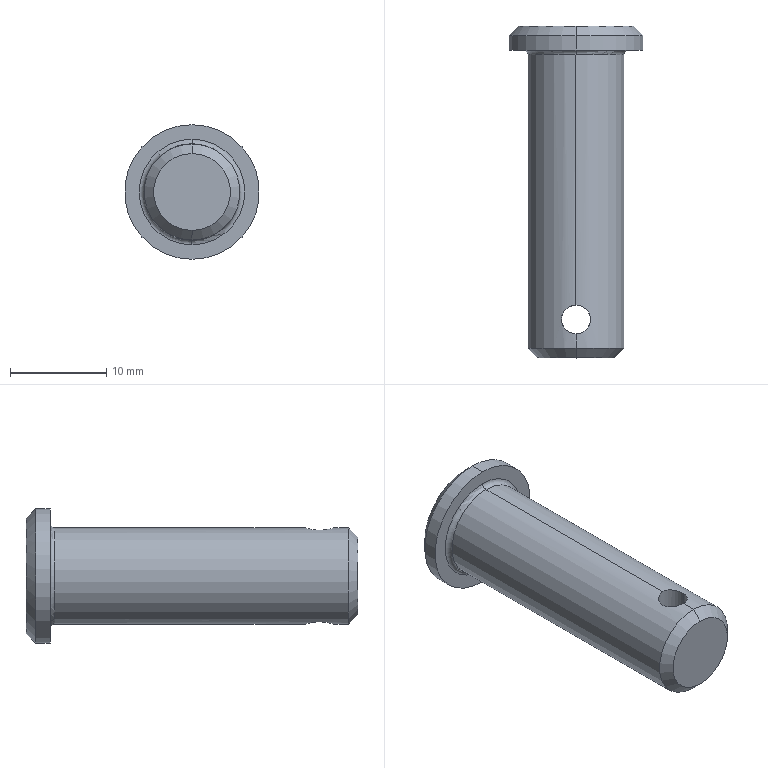Part | SolidWorks | features MirrorStock 1 | 1 solid | 15 faces | box 14 x 34.5 x 14 mm | volume 2794 mm3 | cylinder 6 | cone 4 | plane 3 | torus 2 | commonest cylinder face diameters 3 x2 10 x2 14 x2
STEP:
#1=CARTESIAN_POINT('',(0.,0.,-5.5));
#2=VERTEX_POINT('',#1);
#3=CARTESIAN_POINT('',(0.,0.,5.5));
#4=VERTEX_POINT('',#3);
#5=CARTESIAN_POINT('',(0.,0.,0.));
#6=DIRECTION('',(0.,-1.,0.));
#7=DIRECTION('',(0.,0.,-1.));
#8=AXIS2_PLACEMENT_3D('',#5,#6,#7);
#9=CIRCLE('',#8,5.5);
#10=EDGE_CURVE('',#2,#4,#9,.T.);
#11=ORIENTED_EDGE('',*,*,#10,.T.);
#12=CARTESIAN_POINT('',(0.,-0.5,5.));
#13=VERTEX_POINT('',#12);
#14=CARTESIAN_POINT('',(0.,-0.5,5.5));
#15=DIRECTION('',(-1.,0.,0.));
#16=DIRECTION('',(0.,0.,1.));
#17=AXIS2_PLACEMENT_3D('',#14,#15,#16);
#18=CIRCLE('',#17,0.5);
#19=EDGE_CURVE('',#4,#13,#18,.T.);
#20=ORIENTED_EDGE('',*,*,#19,.T.);
#21=CARTESIAN_POINT('',(0.,-0.5,-5.));
#22=VERTEX_POINT('',#21);
#23=CARTESIAN_POINT('',(0.,-0.5,0.));
#24=DIRECTION('',(0.,1.,0.));
#25=DIRECTION('',(0.,0.,-1.));
#26=AXIS2_PLACEMENT_3D('',#23,#24,#25);
#27=CIRCLE('',#26,5.);
#28=EDGE_CURVE('',#13,#22,#27,.T.);
#29=ORIENTED_EDGE('',*,*,#28,.T.);
#30=CARTESIAN_POINT('',(0.,-0.5,-5.5));
#31=DIRECTION('',(1.,0.,0.));
#32=DIRECTION('',(0.,0.,-1.));
#33=AXIS2_PLACEMENT_3D('',#30,#31,#32);
#34=CIRCLE('',#33,0.5);
#35=EDGE_CURVE('',#2,#22,#34,.T.);
#36=ORIENTED_EDGE('',*,*,#35,.F.);
#37=EDGE_LOOP('',(#11,#20,#29,#36));
#38=FACE_OUTER_BOUND('',#37,.T.);
#39=CARTESIAN_POINT('',(0.,-0.5,0.));
#40=DIRECTION('',(0.,1.,0.));
#41=DIRECTION('',(0.,0.,-1.));
#42=AXIS2_PLACEMENT_3D('',#39,#40,#41);
#43=TOROIDAL_SURFACE('',#42,5.5,0.5);
#44=ADVANCED_FACE('',(#38),#43,.F.);
#45=CARTESIAN_POINT('',(0.,-26.5,5.));
#46=VERTEX_POINT('',#45);
#47=CARTESIAN_POINT('',(-1.5,-28.,4.77));
#48=VERTEX_POINT('',#47);
#49=CARTESIAN_POINT('',(0.,-26.5,5.));
#50=CARTESIAN_POINT('',(-0.09847,-26.5,5.));
#51=CARTESIAN_POINT('',(-0.1985,-26.51,4.997));
#52=CARTESIAN_POINT('',(-0.3913,-26.549,4.986));
#53=CARTESIAN_POINT('',(-0.4851,-26.577,4.977));
#54=CARTESIAN_POINT('',(-0.7586,-26.691,4.946));
#55=CARTESIAN_POINT('',(-0.9231,-26.802,4.916));
#56=CARTESIAN_POINT('',(-1.131,-27.009,4.871));
#57=CARTESIAN_POINT('',(-1.192,-27.084,4.856));
#58=CARTESIAN_POINT('',(-1.301,-27.247,4.828));
#59=CARTESIAN_POINT('',(-1.348,-27.334,4.815));
#60=CARTESIAN_POINT('',(-1.423,-27.515,4.793));
#61=CARTESIAN_POINT('',(-1.451,-27.609,4.785));
#62=CARTESIAN_POINT('',(-1.49,-27.802,4.773));
#63=CARTESIAN_POINT('',(-1.5,-27.902,4.77));
#64=CARTESIAN_POINT('',(-1.5,-28.,4.77));
#65=B_SPLINE_CURVE_WITH_KNOTS('',3,(#49,#50,#51,#52,#53,#54,#55,#56,#57,#58,#59,#60,#61,#62,#63,#64),.UNSPECIFIED.,.F.,.F.,(4,2,2,2,2,2,2,4),(0.002359,0.002654,0.002949,0.003538,0.003833,0.004127,0.004422,0.004717),.UNSPECIFIED.);
#66=EDGE_CURVE('',#46,#48,#65,.T.);
#67=ORIENTED_EDGE('',*,*,#66,.T.);
#68=CARTESIAN_POINT('',(-1.5,-28.,-4.77));
#69=VERTEX_POINT('',#68);
#70=CARTESIAN_POINT('',(-1.5,-28.,7.));
#71=DIRECTION('',(0.,0.,-1.));
#72=VECTOR('',#71,1000.);
#73=LINE('',#70,#72);
#74=EDGE_CURVE('',#48,#69,#73,.T.);
#75=ORIENTED_EDGE('',*,*,#74,.T.);
#76=CARTESIAN_POINT('',(0.,-26.5,-5.));
#77=VERTEX_POINT('',#76);
#78=CARTESIAN_POINT('',(-1.5,-28.,-4.77));
#79=CARTESIAN_POINT('',(-1.5,-27.902,-4.77));
#80=CARTESIAN_POINT('',(-1.49,-27.802,-4.773));
#81=CARTESIAN_POINT('',(-1.451,-27.609,-4.785));
#82=CARTESIAN_POINT('',(-1.423,-27.515,-4.793));
#83=CARTESIAN_POINT('',(-1.309,-27.242,-4.826));
#84=CARTESIAN_POINT('',(-1.199,-27.077,-4.856));
#85=CARTESIAN_POINT('',(-0.9908,-26.87,-4.901));
#86=CARTESIAN_POINT('',(-0.9157,-26.808,-4.916));
#87=CARTESIAN_POINT('',(-0.7536,-26.699,-4.944));
#88=CARTESIAN_POINT('',(-0.6658,-26.652,-4.956));
#89=CARTESIAN_POINT('',(-0.485,-26.577,-4.977));
#90=CARTESIAN_POINT('',(-0.3915,-26.549,-4.986));
#91=CARTESIAN_POINT('',(-0.1977,-26.51,-4.997));
#92=CARTESIAN_POINT('',(-0.09824,-26.5,-5.));
#93=CARTESIAN_POINT('',(0.,-26.5,-5.));
#94=B_SPLINE_CURVE_WITH_KNOTS('',3,(#78,#79,#80,#81,#82,#83,#84,#85,#86,#87,#88,#89,#90,#91,#92,#93),.UNSPECIFIED.,.F.,.F.,(4,2,2,2,2,2,2,4),(0.002359,0.002654,0.002949,0.003538,0.003833,0.004128,0.004422,0.004717),.UNSPECIFIED.);
#95=EDGE_CURVE('',#69,#77,#94,.T.);
#96=ORIENTED_EDGE('',*,*,#95,.T.);
#97=CARTESIAN_POINT('',(1.5,-28.,-4.77));
#98=VERTEX_POINT('',#97);
#99=CARTESIAN_POINT('',(0.,-26.5,-5.));
#100=CARTESIAN_POINT('',(0.1965,-26.5,-5.));
#101=CARTESIAN_POINT('',(0.3949,-26.54,-4.988));
#102=CARTESIAN_POINT('',(0.6662,-26.652,-4.956));
#103=CARTESIAN_POINT('',(0.7539,-26.7,-4.944));
#104=CARTESIAN_POINT('',(0.9162,-26.808,-4.916));
#105=CARTESIAN_POINT('',(0.9914,-26.87,-4.901));
#106=CARTESIAN_POINT('',(1.199,-27.078,-4.856));
#107=CARTESIAN_POINT('',(1.309,-27.241,-4.826));
#108=CARTESIAN_POINT('',(1.423,-27.515,-4.793));
#109=CARTESIAN_POINT('',(1.452,-27.609,-4.785));
#110=CARTESIAN_POINT('',(1.49,-27.801,-4.773));
#111=CARTESIAN_POINT('',(1.5,-27.901,-4.77));
#112=CARTESIAN_POINT('',(1.5,-28.,-4.77));
#113=B_SPLINE_CURVE_WITH_KNOTS('',3,(#99,#100,#101,#102,#103,#104,#105,#106,#107,#108,#109,#110,#111,#112),.UNSPECIFIED.,.F.,.F.,(4,2,2,2,2,2,4),(0.004717,0.005306,0.005601,0.005896,0.006485,0.00678,0.007075),.UNSPECIFIED.);
#114=EDGE_CURVE('',#77,#98,#113,.T.);
#115=ORIENTED_EDGE('',*,*,#114,.T.);
#116=CARTESIAN_POINT('',(1.5,-28.,4.77));
#117=VERTEX_POINT('',#116);
#118=CARTESIAN_POINT('',(1.5,-28.,7.));
#119=DIRECTION('',(0.,0.,-1.));
#120=VECTOR('',#119,1000.);
#121=LINE('',#118,#120);
#122=EDGE_CURVE('',#117,#98,#121,.T.);
#123=ORIENTED_EDGE('',*,*,#122,.F.);
#124=CARTESIAN_POINT('',(1.5,-28.,4.77));
#125=CARTESIAN_POINT('',(1.5,-27.9,4.77));
#126=CARTESIAN_POINT('',(1.49,-27.802,4.773));
#127=CARTESIAN_POINT('',(1.452,-27.61,4.785));
#128=CARTESIAN_POINT('',(1.423,-27.514,4.794));
#129=CARTESIAN_POINT('',(1.347,-27.333,4.815));
#130=CARTESIAN_POINT('',(1.301,-27.247,4.828));
#131=CARTESIAN_POINT('',(1.192,-27.084,4.856));
#132=CARTESIAN_POINT('',(1.129,-27.008,4.871));
#133=CARTESIAN_POINT('',(0.9226,-26.801,4.916));
#134=CARTESIAN_POINT('',(0.7561,-26.69,4.946));
#135=CARTESIAN_POINT('',(0.3953,-26.54,4.988));
#136=CARTESIAN_POINT('',(0.197,-26.5,5.));
#137=CARTESIAN_POINT('',(0.,-26.5,5.));
#138=B_SPLINE_CURVE_WITH_KNOTS('',3,(#124,#125,#126,#127,#128,#129,#130,#131,#132,#133,#134,#135,#136,#137),.UNSPECIFIED.,.F.,.F.,(4,2,2,2,2,2,4),(0.,0.0002949,0.0005898,0.0008847,0.00118,0.001769,0.002359),.UNSPECIFIED.);
#139=EDGE_CURVE('',#117,#46,#138,.T.);
#140=ORIENTED_EDGE('',*,*,#139,.T.);
#141=EDGE_LOOP('',(#67,#75,#96,#115,#123,#140));
#142=FACE_OUTER_BOUND('',#141,.T.);
#143=CARTESIAN_POINT('',(0.,-28.,7.));
#144=DIRECTION('',(0.,0.,-1.));
#145=DIRECTION('',(1.,0.,0.));
#146=AXIS2_PLACEMENT_3D('',#143,#144,#145);
#147=CYLINDRICAL_SURFACE('',#146,1.5);
#148=ADVANCED_FACE('',(#142),#147,.F.);
#149=CARTESIAN_POINT('',(0.,2.5,6.));
#150=VERTEX_POINT('',#149);
#151=CARTESIAN_POINT('',(0.,2.5,-6.));
#152=VERTEX_POINT('',#151);
#153=CARTESIAN_POINT('',(0.,2.5,0.));
#154=DIRECTION('',(0.,-1.,0.));
#155=DIRECTION('',(0.,0.,-1.));
#156=AXIS2_PLACEMENT_3D('',#153,#154,#155);
#157=CIRCLE('',#156,6.);
#158=EDGE_CURVE('',#150,#152,#157,.T.);
#159=ORIENTED_EDGE('',*,*,#158,.T.);
#160=CARTESIAN_POINT('',(0.,1.5,-7.));
#161=VERTEX_POINT('',#160);
#162=CARTESIAN_POINT('',(0.,2.5,-6.));
#163=DIRECTION('',(0.,-0.7071,-0.7071));
#164=VECTOR('',#163,1000.);
#165=LINE('',#162,#164);
#166=EDGE_CURVE('',#152,#161,#165,.T.);
#167=ORIENTED_EDGE('',*,*,#166,.T.);
#168=CARTESIAN_POINT('',(0.,1.5,7.));
#169=VERTEX_POINT('',#168);
#170=CARTESIAN_POINT('',(0.,1.5,0.));
#171=DIRECTION('',(0.,1.,0.));
#172=DIRECTION('',(0.,0.,-1.));
#173=AXIS2_PLACEMENT_3D('',#170,#171,#172);
#174=CIRCLE('',#173,7.);
#175=EDGE_CURVE('',#161,#169,#174,.T.);
#176=ORIENTED_EDGE('',*,*,#175,.T.);
#177=CARTESIAN_POINT('',(0.,2.5,6.));
#178=DIRECTION('',(0.,-0.7071,0.7071));
#179=VECTOR('',#178,1000.);
#180=LINE('',#177,#179);
#181=EDGE_CURVE('',#150,#169,#180,.T.);
#182=ORIENTED_EDGE('',*,*,#181,.F.);
#183=EDGE_LOOP('',(#159,#167,#176,#182));
#184=FACE_OUTER_BOUND('',#183,.T.);
#185=CARTESIAN_POINT('',(0.,2.5,0.));
#186=DIRECTION('',(0.,-1.,0.));
#187=DIRECTION('',(0.,0.,1.));
#188=AXIS2_PLACEMENT_3D('',#185,#186,#187);
#189=CONICAL_SURFACE('',#188,6.,0.7854);
#190=ADVANCED_FACE('',(#184),#189,.T.);
#191=CARTESIAN_POINT('',(0.,-32.,-4.));
#192=VERTEX_POINT('',#191);
#193=CARTESIAN_POINT('',(0.,-32.,4.));
#194=VERTEX_POINT('',#193);
#195=CARTESIAN_POINT('',(0.,-32.,0.));
#196=DIRECTION('',(0.,1.,0.));
#197=DIRECTION('',(0.,0.,1.));
#198=AXIS2_PLACEMENT_3D('',#195,#196,#197);
#199=CIRCLE('',#198,4.);
#200=EDGE_CURVE('',#192,#194,#199,.T.);
#201=ORIENTED_EDGE('',*,*,#200,.T.);
#202=CARTESIAN_POINT('',(0.,-31.,5.));
#203=VERTEX_POINT('',#202);
#204=CARTESIAN_POINT('',(0.,-32.,4.));
#205=DIRECTION('',(0.,0.7071,0.7071));
#206=VECTOR('',#205,1000.);
#207=LINE('',#204,#206);
#208=EDGE_CURVE('',#194,#203,#207,.T.);
#209=ORIENTED_EDGE('',*,*,#208,.T.);
#210=CARTESIAN_POINT('',(0.,-31.,-5.));
#211=VERTEX_POINT('',#210);
#212=CARTESIAN_POINT('',(0.,-31.,0.));
#213=DIRECTION('',(0.,-1.,0.));
#214=DIRECTION('',(0.,0.,1.));
#215=AXIS2_PLACEMENT_3D('',#212,#213,#214);
#216=CIRCLE('',#215,5.);
#217=EDGE_CURVE('',#203,#211,#216,.T.);
#218=ORIENTED_EDGE('',*,*,#217,.T.);
#219=CARTESIAN_POINT('',(0.,-32.,-4.));
#220=DIRECTION('',(0.,0.7071,-0.7071));
#221=VECTOR('',#220,1000.);
#222=LINE('',#219,#221);
#223=EDGE_CURVE('',#192,#211,#222,.T.);
#224=ORIENTED_EDGE('',*,*,#223,.F.);
#225=EDGE_LOOP('',(#201,#209,#218,#224));
#226=FACE_OUTER_BOUND('',#225,.T.);
#227=CARTESIAN_POINT('',(0.,-32.,0.));
#228=DIRECTION('',(0.,1.,0.));
#229=DIRECTION('',(0.,0.,-1.));
#230=AXIS2_PLACEMENT_3D('',#227,#228,#229);
#231=CONICAL_SURFACE('',#230,4.,0.7854);
#232=ADVANCED_FACE('',(#226),#231,.T.);
#233=ORIENTED_EDGE('',*,*,#217,.F.);
#234=CARTESIAN_POINT('',(0.,-29.5,5.));
#235=VERTEX_POINT('',#234);
#236=CARTESIAN_POINT('',(0.,-32.,5.));
#237=DIRECTION('',(0.,1.,0.));
#238=VECTOR('',#237,1000.);
#239=LINE('',#236,#238);
#240=EDGE_CURVE('',#203,#235,#239,.T.);
#241=ORIENTED_EDGE('',*,*,#240,.T.);
#242=CARTESIAN_POINT('',(-1.5,-28.,4.77));
#243=CARTESIAN_POINT('',(-1.5,-28.196,4.77));
#244=CARTESIAN_POINT('',(-1.46,-28.395,4.783));
#245=CARTESIAN_POINT('',(-1.348,-28.666,4.815));
#246=CARTESIAN_POINT('',(-1.301,-28.754,4.828));
#247=CARTESIAN_POINT('',(-1.192,-28.916,4.856));
#248=CARTESIAN_POINT('',(-1.13,-28.991,4.871));
#249=CARTESIAN_POINT('',(-0.9225,-29.199,4.916));
#250=CARTESIAN_POINT('',(-0.759,-29.309,4.945));
#251=CARTESIAN_POINT('',(-0.4847,-29.423,4.977));
#252=CARTESIAN_POINT('',(-0.3908,-29.452,4.986));
#253=CARTESIAN_POINT('',(-0.1985,-29.49,4.997));
#254=CARTESIAN_POINT('',(-0.09886,-29.5,5.));
#255=CARTESIAN_POINT('',(0.,-29.5,5.));
#256=B_SPLINE_CURVE_WITH_KNOTS('',3,(#242,#243,#244,#245,#246,#247,#248,#249,#250,#251,#252,#253,#254,#255),.UNSPECIFIED.,.F.,.F.,(4,2,2,2,2,2,4),(0.004717,0.005306,0.005601,0.005896,0.006485,0.00678,0.007075),.UNSPECIFIED.);
#257=EDGE_CURVE('',#48,#235,#256,.T.);
#258=ORIENTED_EDGE('',*,*,#257,.F.);
#259=ORIENTED_EDGE('',*,*,#66,.F.);
#260=CARTESIAN_POINT('',(0.,-32.,5.));
#261=DIRECTION('',(0.,1.,0.));
#262=VECTOR('',#261,1000.);
#263=LINE('',#260,#262);
#264=EDGE_CURVE('',#46,#13,#263,.T.);
#265=ORIENTED_EDGE('',*,*,#264,.T.);
#266=CARTESIAN_POINT('',(0.,-0.5,0.));
#267=DIRECTION('',(0.,1.,0.));
#268=DIRECTION('',(0.,0.,-1.));
#269=AXIS2_PLACEMENT_3D('',#266,#267,#268);
#270=CIRCLE('',#269,5.);
#271=EDGE_CURVE('',#22,#13,#270,.T.);
#272=ORIENTED_EDGE('',*,*,#271,.F.);
#273=CARTESIAN_POINT('',(0.,-32.,-5.));
#274=DIRECTION('',(0.,1.,0.));
#275=VECTOR('',#274,1000.);
#276=LINE('',#273,#275);
#277=EDGE_CURVE('',#77,#22,#276,.T.);
#278=ORIENTED_EDGE('',*,*,#277,.F.);
#279=ORIENTED_EDGE('',*,*,#95,.F.);
#280=CARTESIAN_POINT('',(0.,-29.5,-5.));
#281=VERTEX_POINT('',#280);
#282=CARTESIAN_POINT('',(0.,-29.5,-5.));
#283=CARTESIAN_POINT('',(-0.09976,-29.5,-5.));
#284=CARTESIAN_POINT('',(-0.1977,-29.49,-4.997));
#285=CARTESIAN_POINT('',(-0.3903,-29.452,-4.986));
#286=CARTESIAN_POINT('',(-0.4859,-29.423,-4.977));
#287=CARTESIAN_POINT('',(-0.6674,-29.347,-4.956));
#288=CARTESIAN_POINT('',(-0.7534,-29.301,-4.944));
#289=CARTESIAN_POINT('',(-0.916,-29.192,-4.916));
#290=CARTESIAN_POINT('',(-0.9926,-29.129,-4.901));
#291=CARTESIAN_POINT('',(-1.199,-28.922,-4.856));
#292=CARTESIAN_POINT('',(-1.31,-28.756,-4.826));
#293=CARTESIAN_POINT('',(-1.46,-28.395,-4.783));
#294=CARTESIAN_POINT('',(-1.5,-28.197,-4.77));
#295=CARTESIAN_POINT('',(-1.5,-28.,-4.77));
#296=B_SPLINE_CURVE_WITH_KNOTS('',3,(#282,#283,#284,#285,#286,#287,#288,#289,#290,#291,#292,#293,#294,#295),.UNSPECIFIED.,.F.,.F.,(4,2,2,2,2,2,4),(0.,0.0002949,0.0005898,0.0008847,0.00118,0.001769,0.002359),.UNSPECIFIED.);
#297=EDGE_CURVE('',#281,#69,#296,.T.);
#298=ORIENTED_EDGE('',*,*,#297,.F.);
#299=CARTESIAN_POINT('',(0.,-32.,-5.));
#300=DIRECTION('',(0.,1.,0.));
#301=VECTOR('',#300,1000.);
#302=LINE('',#299,#301);
#303=EDGE_CURVE('',#211,#281,#302,.T.);
#304=ORIENTED_EDGE('',*,*,#303,.F.);
#305=EDGE_LOOP('',(#233,#241,#258,#259,#265,#272,#278,#279,#298,#304));
#306=FACE_OUTER_BOUND('',#305,.T.);
#307=CARTESIAN_POINT('',(0.,-32.,0.));
#308=DIRECTION('',(0.,1.,0.));
#309=DIRECTION('',(0.,0.,-1.));
#310=AXIS2_PLACEMENT_3D('',#307,#308,#309);
#311=CYLINDRICAL_SURFACE('',#310,5.);
#312=ADVANCED_FACE('',(#306),#311,.T.);
#313=ORIENTED_EDGE('',*,*,#175,.F.);
#314=CARTESIAN_POINT('',(0.,0.,-7.));
#315=VERTEX_POINT('',#314);
#316=CARTESIAN_POINT('',(0.,2.5,-7.));
#317=DIRECTION('',(0.,-1.,0.));
#318=VECTOR('',#317,1000.);
#319=LINE('',#316,#318);
#320=EDGE_CURVE('',#161,#315,#319,.T.);
#321=ORIENTED_EDGE('',*,*,#320,.T.);
#322=CARTESIAN_POINT('',(0.,0.,7.));
#323=VERTEX_POINT('',#322);
#324=CARTESIAN_POINT('',(0.,0.,0.));
#325=DIRECTION('',(0.,-1.,0.));
#326=DIRECTION('',(0.,0.,-1.));
#327=AXIS2_PLACEMENT_3D('',#324,#325,#326);
#328=CIRCLE('',#327,7.);
#329=EDGE_CURVE('',#323,#315,#328,.T.);
#330=ORIENTED_EDGE('',*,*,#329,.F.);
#331=CARTESIAN_POINT('',(0.,2.5,7.));
#332=DIRECTION('',(0.,-1.,0.));
#333=VECTOR('',#332,1000.);
#334=LINE('',#331,#333);
#335=EDGE_CURVE('',#169,#323,#334,.T.);
#336=ORIENTED_EDGE('',*,*,#335,.F.);
#337=EDGE_LOOP('',(#313,#321,#330,#336));
#338=FACE_OUTER_BOUND('',#337,.T.);
#339=CARTESIAN_POINT('',(0.,2.5,0.));
#340=DIRECTION('',(0.,-1.,0.));
#341=DIRECTION('',(0.,0.,1.));
#342=AXIS2_PLACEMENT_3D('',#339,#340,#341);
#343=CYLINDRICAL_SURFACE('',#342,7.);
#344=ADVANCED_FACE('',(#338),#343,.T.);
#345=ORIENTED_EDGE('',*,*,#320,.F.);
#346=CARTESIAN_POINT('',(0.,1.5,0.));
#347=DIRECTION('',(0.,1.,0.));
#348=DIRECTION('',(0.,0.,-1.));
#349=AXIS2_PLACEMENT_3D('',#346,#347,#348);
#350=CIRCLE('',#349,7.);
#351=EDGE_CURVE('',#169,#161,#350,.T.);
#352=ORIENTED_EDGE('',*,*,#351,.F.);
#353=ORIENTED_EDGE('',*,*,#335,.T.);
#354=CARTESIAN_POINT('',(0.,0.,0.));
#355=DIRECTION('',(0.,-1.,0.));
#356=DIRECTION('',(0.,0.,-1.));
#357=AXIS2_PLACEMENT_3D('',#354,#355,#356);
#358=CIRCLE('',#357,7.);
#359=EDGE_CURVE('',#315,#323,#358,.T.);
#360=ORIENTED_EDGE('',*,*,#359,.F.);
#361=EDGE_LOOP('',(#345,#352,#353,#360));
#362=FACE_OUTER_BOUND('',#361,.T.);
#363=CARTESIAN_POINT('',(0.,2.5,0.));
#364=DIRECTION('',(0.,-1.,0.));
#365=DIRECTION('',(0.,0.,1.));
#366=AXIS2_PLACEMENT_3D('',#363,#364,#365);
#367=CYLINDRICAL_SURFACE('',#366,7.);
#368=ADVANCED_FACE('',(#362),#367,.T.);
#369=ORIENTED_EDGE('',*,*,#158,.F.);
#370=CARTESIAN_POINT('',(0.,2.5,0.));
#371=DIRECTION('',(0.,-1.,0.));
#372=DIRECTION('',(0.,0.,-1.));
#373=AXIS2_PLACEMENT_3D('',#370,#371,#372);
#374=CIRCLE('',#373,6.);
#375=EDGE_CURVE('',#152,#150,#374,.T.);
#376=ORIENTED_EDGE('',*,*,#375,.F.);
#377=EDGE_LOOP('',(#369,#376));
#378=FACE_OUTER_BOUND('',#377,.T.);
#379=CARTESIAN_POINT('',(0.,2.5,0.));
#380=DIRECTION('',(0.,1.,0.));
#381=DIRECTION('',(0.,0.,-1.));
#382=AXIS2_PLACEMENT_3D('',#379,#380,#381);
#383=PLANE('',#382);
#384=ADVANCED_FACE('',(#378),#383,.T.);
#385=ORIENTED_EDGE('',*,*,#10,.F.);
#386=CARTESIAN_POINT('',(0.,0.,0.));
#387=DIRECTION('',(0.,-1.,0.));
#388=DIRECTION('',(0.,0.,-1.));
#389=AXIS2_PLACEMENT_3D('',#386,#387,#388);
#390=CIRCLE('',#389,5.5);
#391=EDGE_CURVE('',#4,#2,#390,.T.);
#392=ORIENTED_EDGE('',*,*,#391,.F.);
#393=EDGE_LOOP('',(#385,#392));
#394=FACE_BOUND('',#393,.T.);
#395=ORIENTED_EDGE('',*,*,#329,.T.);
#396=ORIENTED_EDGE('',*,*,#359,.T.);
#397=EDGE_LOOP('',(#395,#396));
#398=FACE_OUTER_BOUND('',#397,.T.);
#399=CARTESIAN_POINT('',(0.,0.,0.));
#400=DIRECTION('',(0.,1.,0.));
#401=DIRECTION('',(0.,0.,-1.));
#402=AXIS2_PLACEMENT_3D('',#399,#400,#401);
#403=PLANE('',#402);
#404=ADVANCED_FACE('',(#394,#398),#403,.F.);
#405=ORIENTED_EDGE('',*,*,#240,.F.);
#406=CARTESIAN_POINT('',(0.,-31.,0.));
#407=DIRECTION('',(0.,-1.,0.));
#408=DIRECTION('',(0.,0.,1.));
#409=AXIS2_PLACEMENT_3D('',#406,#407,#408);
#410=CIRCLE('',#409,5.);
#411=EDGE_CURVE('',#211,#203,#410,.T.);
#412=ORIENTED_EDGE('',*,*,#411,.F.);
#413=ORIENTED_EDGE('',*,*,#303,.T.);
#414=CARTESIAN_POINT('',(1.5,-28.,-4.77));
#415=CARTESIAN_POINT('',(1.5,-28.099,-4.77));
#416=CARTESIAN_POINT('',(1.49,-28.197,-4.773));
#417=CARTESIAN_POINT('',(1.452,-28.39,-4.785));
#418=CARTESIAN_POINT('',(1.423,-28.486,-4.794));
#419=CARTESIAN_POINT('',(1.31,-28.757,-4.826));
#420=CARTESIAN_POINT('',(1.198,-28.923,-4.856));
#421=CARTESIAN_POINT('',(0.9923,-29.129,-4.901));
#422=CARTESIAN_POINT('',(0.9158,-29.192,-4.916));
#423=CARTESIAN_POINT('',(0.7532,-29.301,-4.944));
#424=CARTESIAN_POINT('',(0.6674,-29.347,-4.956));
#425=CARTESIAN_POINT('',(0.4865,-29.422,-4.977));
#426=CARTESIAN_POINT('',(0.3907,-29.452,-4.986));
#427=CARTESIAN_POINT('',(0.1978,-29.49,-4.997));
#428=CARTESIAN_POINT('',(0.0997,-29.5,-5.));
#429=CARTESIAN_POINT('',(0.,-29.5,-5.));
#430=B_SPLINE_CURVE_WITH_KNOTS('',3,(#414,#415,#416,#417,#418,#419,#420,#421,#422,#423,#424,#425,#426,#427,#428,#429),.UNSPECIFIED.,.F.,.F.,(4,2,2,2,2,2,2,4),(0.007075,0.00737,0.007664,0.008254,0.008549,0.008843,0.009138,0.009433),.UNSPECIFIED.);
#431=EDGE_CURVE('',#98,#281,#430,.T.);
#432=ORIENTED_EDGE('',*,*,#431,.F.);
#433=ORIENTED_EDGE('',*,*,#114,.F.);
#434=ORIENTED_EDGE('',*,*,#277,.T.);
#435=ORIENTED_EDGE('',*,*,#28,.F.);
#436=ORIENTED_EDGE('',*,*,#264,.F.);
#437=ORIENTED_EDGE('',*,*,#139,.F.);
#438=CARTESIAN_POINT('',(0.,-29.5,5.));
#439=CARTESIAN_POINT('',(0.09885,-29.5,5.));
#440=CARTESIAN_POINT('',(0.1966,-29.49,4.997));
#441=CARTESIAN_POINT('',(0.3899,-29.452,4.986));
#442=CARTESIAN_POINT('',(0.4856,-29.423,4.977));
#443=CARTESIAN_POINT('',(0.7566,-29.31,4.946));
#444=CARTESIAN_POINT('',(0.9229,-29.198,4.916));
#445=CARTESIAN_POINT('',(1.129,-28.992,4.871));
#446=CARTESIAN_POINT('',(1.192,-28.916,4.856));
#447=CARTESIAN_POINT('',(1.301,-28.753,4.828));
#448=CARTESIAN_POINT('',(1.347,-28.667,4.815));
#449=CARTESIAN_POINT('',(1.422,-28.486,4.794));
#450=CARTESIAN_POINT('',(1.452,-28.391,4.785));
#451=CARTESIAN_POINT('',(1.49,-28.198,4.773));
#452=CARTESIAN_POINT('',(1.5,-28.1,4.77));
#453=CARTESIAN_POINT('',(1.5,-28.,4.77));
#454=B_SPLINE_CURVE_WITH_KNOTS('',3,(#438,#439,#440,#441,#442,#443,#444,#445,#446,#447,#448,#449,#450,#451,#452,#453),.UNSPECIFIED.,.F.,.F.,(4,2,2,2,2,2,2,4),(0.007075,0.00737,0.007664,0.008254,0.008548,0.008843,0.009138,0.009433),.UNSPECIFIED.);
#455=EDGE_CURVE('',#235,#117,#454,.T.);
#456=ORIENTED_EDGE('',*,*,#455,.F.);
#457=EDGE_LOOP('',(#405,#412,#413,#432,#433,#434,#435,#436,#437,#456));
#458=FACE_OUTER_BOUND('',#457,.T.);
#459=CARTESIAN_POINT('',(0.,-32.,0.));
#460=DIRECTION('',(0.,1.,0.));
#461=DIRECTION('',(0.,0.,-1.));
#462=AXIS2_PLACEMENT_3D('',#459,#460,#461);
#463=CYLINDRICAL_SURFACE('',#462,5.);
#464=ADVANCED_FACE('',(#458),#463,.T.);
#465=ORIENTED_EDGE('',*,*,#200,.F.);
#466=CARTESIAN_POINT('',(0.,-32.,0.));
#467=DIRECTION('',(0.,1.,0.));
#468=DIRECTION('',(0.,0.,1.));
#469=AXIS2_PLACEMENT_3D('',#466,#467,#468);
#470=CIRCLE('',#469,4.);
#471=EDGE_CURVE('',#194,#192,#470,.T.);
#472=ORIENTED_EDGE('',*,*,#471,.F.);
#473=EDGE_LOOP('',(#465,#472));
#474=FACE_OUTER_BOUND('',#473,.T.);
#475=CARTESIAN_POINT('',(0.,-32.,0.));
#476=DIRECTION('',(0.,-1.,0.));
#477=DIRECTION('',(0.,0.,1.));
#478=AXIS2_PLACEMENT_3D('',#475,#476,#477);
#479=PLANE('',#478);
#480=ADVANCED_FACE('',(#474),#479,.T.);
#481=ORIENTED_EDGE('',*,*,#208,.F.);
#482=ORIENTED_EDGE('',*,*,#471,.T.);
#483=ORIENTED_EDGE('',*,*,#223,.T.);
#484=ORIENTED_EDGE('',*,*,#411,.T.);
#485=EDGE_LOOP('',(#481,#482,#483,#484));
#486=FACE_OUTER_BOUND('',#485,.T.);
#487=CARTESIAN_POINT('',(0.,-32.,0.));
#488=DIRECTION('',(0.,1.,0.));
#489=DIRECTION('',(0.,0.,-1.));
#490=AXIS2_PLACEMENT_3D('',#487,#488,#489);
#491=CONICAL_SURFACE('',#490,4.,0.7854);
#492=ADVANCED_FACE('',(#486),#491,.T.);
#493=ORIENTED_EDGE('',*,*,#166,.F.);
#494=ORIENTED_EDGE('',*,*,#375,.T.);
#495=ORIENTED_EDGE('',*,*,#181,.T.);
#496=ORIENTED_EDGE('',*,*,#351,.T.);
#497=EDGE_LOOP('',(#493,#494,#495,#496));
#498=FACE_OUTER_BOUND('',#497,.T.);
#499=CARTESIAN_POINT('',(0.,2.5,0.));
#500=DIRECTION('',(0.,-1.,0.));
#501=DIRECTION('',(0.,0.,1.));
#502=AXIS2_PLACEMENT_3D('',#499,#500,#501);
#503=CONICAL_SURFACE('',#502,6.,0.7854);
#504=ADVANCED_FACE('',(#498),#503,.T.);
#505=ORIENTED_EDGE('',*,*,#74,.F.);
#506=ORIENTED_EDGE('',*,*,#257,.T.);
#507=ORIENTED_EDGE('',*,*,#455,.T.);
#508=ORIENTED_EDGE('',*,*,#122,.T.);
#509=ORIENTED_EDGE('',*,*,#431,.T.);
#510=ORIENTED_EDGE('',*,*,#297,.T.);
#511=EDGE_LOOP('',(#505,#506,#507,#508,#509,#510));
#512=FACE_OUTER_BOUND('',#511,.T.);
#513=CARTESIAN_POINT('',(0.,-28.,7.));
#514=DIRECTION('',(0.,0.,-1.));
#515=DIRECTION('',(1.,0.,0.));
#516=AXIS2_PLACEMENT_3D('',#513,#514,#515);
#517=CYLINDRICAL_SURFACE('',#516,1.5);
#518=ADVANCED_FACE('',(#512),#517,.F.);
#519=ORIENTED_EDGE('',*,*,#19,.F.);
#520=ORIENTED_EDGE('',*,*,#391,.T.);
#521=ORIENTED_EDGE('',*,*,#35,.T.);
#522=ORIENTED_EDGE('',*,*,#271,.T.);
#523=EDGE_LOOP('',(#519,#520,#521,#522));
#524=FACE_OUTER_BOUND('',#523,.T.);
#525=CARTESIAN_POINT('',(0.,-0.5,0.));
#526=DIRECTION('',(0.,1.,0.));
#527=DIRECTION('',(0.,0.,-1.));
#528=AXIS2_PLACEMENT_3D('',#525,#526,#527);
#529=TOROIDAL_SURFACE('',#528,5.5,0.5);
#530=ADVANCED_FACE('',(#524),#529,.F.);
#531=CLOSED_SHELL('',(#44,#148,#190,#232,#312,#344,#368,#384,#404,#464,#480,#492,#504,#518,#530));
#532=MANIFOLD_SOLID_BREP('',#531);
#533=CARTESIAN_POINT('',(0.,0.,0.));
#534=DIRECTION('',(0.,0.,1.));
#535=DIRECTION('',(1.,0.,0.));
#536=AXIS2_PLACEMENT_3D('',#533,#534,#535);
#537=(LENGTH_UNIT()NAMED_UNIT(*)SI_UNIT(.MILLI.,.METRE.));
#538=UNCERTAINTY_MEASURE_WITH_UNIT(LENGTH_MEASURE(0.00001),#537,'','');
#539=(NAMED_UNIT(*)PLANE_ANGLE_UNIT()SI_UNIT($,.RADIAN.));
#540=(NAMED_UNIT(*)SI_UNIT($,.STERADIAN.)SOLID_ANGLE_UNIT());
#541=(GEOMETRIC_REPRESENTATION_CONTEXT(3)GLOBAL_UNCERTAINTY_ASSIGNED_CONTEXT((#538))GLOBAL_UNIT_ASSIGNED_CONTEXT((#537,#539,#540))REPRESENTATION_CONTEXT('',''));
#542=ADVANCED_BREP_SHAPE_REPRESENTATION('',(#532,#536),#541);